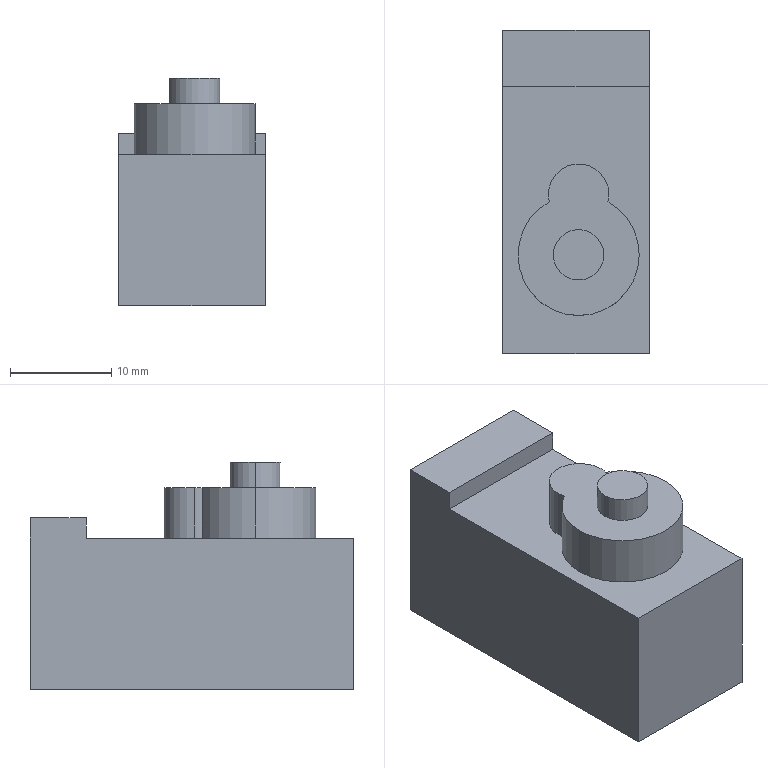Part | SolidWorks | features BaseBody 1 | 1 solid | 18 faces | box 14.483 x 32 x 22.5 mm | volume 7805 mm3 | plane 10 | cylinder 8 | commonest cylinder face diameters 6 x3 12 x3 5 x2
STEP:
#1=CARTESIAN_POINT('',(4.506,-11.764,22.5));
#2=VERTEX_POINT('',#1);
#3=CARTESIAN_POINT('',(-0.4937,-11.764,22.5));
#4=VERTEX_POINT('',#3);
#5=CARTESIAN_POINT('',(2.006,-11.764,22.5));
#6=DIRECTION('',(0.,0.,1.));
#7=DIRECTION('',(1.,0.,0.));
#8=AXIS2_PLACEMENT_3D('',#5,#6,#7);
#9=CIRCLE('',#8,2.5);
#10=EDGE_CURVE('',#2,#4,#9,.T.);
#11=ORIENTED_EDGE('',*,*,#10,.F.);
#12=CARTESIAN_POINT('',(4.506,-11.764,20.));
#13=VERTEX_POINT('',#12);
#14=CARTESIAN_POINT('',(4.506,-11.764,22.5));
#15=DIRECTION('',(0.,0.,-1.));
#16=VECTOR('',#15,1000.);
#17=LINE('',#14,#16);
#18=EDGE_CURVE('',#2,#13,#17,.T.);
#19=ORIENTED_EDGE('',*,*,#18,.T.);
#20=CARTESIAN_POINT('',(-0.4937,-11.764,20.));
#21=VERTEX_POINT('',#20);
#22=CARTESIAN_POINT('',(2.006,-11.764,20.));
#23=DIRECTION('',(0.,0.,1.));
#24=DIRECTION('',(1.,0.,0.));
#25=AXIS2_PLACEMENT_3D('',#22,#23,#24);
#26=CIRCLE('',#25,2.5);
#27=EDGE_CURVE('',#13,#21,#26,.T.);
#28=ORIENTED_EDGE('',*,*,#27,.T.);
#29=CARTESIAN_POINT('',(-0.4937,-11.764,22.5));
#30=DIRECTION('',(0.,0.,-1.));
#31=VECTOR('',#30,1000.);
#32=LINE('',#29,#31);
#33=EDGE_CURVE('',#4,#21,#32,.T.);
#34=ORIENTED_EDGE('',*,*,#33,.F.);
#35=EDGE_LOOP('',(#11,#19,#28,#34));
#36=FACE_OUTER_BOUND('',#35,.T.);
#37=CARTESIAN_POINT('',(2.006,-11.764,22.5));
#38=DIRECTION('',(0.,0.,-1.));
#39=DIRECTION('',(-1.,0.,0.));
#40=AXIS2_PLACEMENT_3D('',#37,#38,#39);
#41=CYLINDRICAL_SURFACE('',#40,2.5);
#42=ADVANCED_FACE('',(#36),#41,.T.);
#43=CARTESIAN_POINT('',(8.006,-11.764,20.));
#44=VERTEX_POINT('',#43);
#45=CARTESIAN_POINT('',(4.911,-6.514,20.));
#46=VERTEX_POINT('',#45);
#47=CARTESIAN_POINT('',(2.006,-11.764,20.));
#48=DIRECTION('',(0.,0.,1.));
#49=DIRECTION('',(1.,0.,0.));
#50=AXIS2_PLACEMENT_3D('',#47,#48,#49);
#51=CIRCLE('',#50,6.);
#52=EDGE_CURVE('',#44,#46,#51,.T.);
#53=ORIENTED_EDGE('',*,*,#52,.F.);
#54=CARTESIAN_POINT('',(8.006,-11.764,15.));
#55=VERTEX_POINT('',#54);
#56=CARTESIAN_POINT('',(8.006,-11.764,20.));
#57=DIRECTION('',(0.,0.,-1.));
#58=VECTOR('',#57,1000.);
#59=LINE('',#56,#58);
#60=EDGE_CURVE('',#44,#55,#59,.T.);
#61=ORIENTED_EDGE('',*,*,#60,.T.);
#62=CARTESIAN_POINT('',(4.911,-6.514,15.));
#63=VERTEX_POINT('',#62);
#64=CARTESIAN_POINT('',(2.006,-11.764,15.));
#65=DIRECTION('',(0.,0.,1.));
#66=DIRECTION('',(1.,0.,0.));
#67=AXIS2_PLACEMENT_3D('',#64,#65,#66);
#68=CIRCLE('',#67,6.);
#69=EDGE_CURVE('',#55,#63,#68,.T.);
#70=ORIENTED_EDGE('',*,*,#69,.T.);
#71=CARTESIAN_POINT('',(4.911,-6.514,20.));
#72=DIRECTION('',(0.,0.,-1.));
#73=VECTOR('',#72,1000.);
#74=LINE('',#71,#73);
#75=EDGE_CURVE('',#46,#63,#74,.T.);
#76=ORIENTED_EDGE('',*,*,#75,.F.);
#77=EDGE_LOOP('',(#53,#61,#70,#76));
#78=FACE_OUTER_BOUND('',#77,.T.);
#79=CARTESIAN_POINT('',(2.006,-11.764,20.));
#80=DIRECTION('',(0.,0.,-1.));
#81=DIRECTION('',(-1.,0.,0.));
#82=AXIS2_PLACEMENT_3D('',#79,#80,#81);
#83=CYLINDRICAL_SURFACE('',#82,6.);
#84=ADVANCED_FACE('',(#78),#83,.T.);
#85=ORIENTED_EDGE('',*,*,#60,.F.);
#86=CARTESIAN_POINT('',(-3.994,-11.764,20.));
#87=VERTEX_POINT('',#86);
#88=CARTESIAN_POINT('',(2.006,-11.764,20.));
#89=DIRECTION('',(0.,0.,1.));
#90=DIRECTION('',(1.,0.,0.));
#91=AXIS2_PLACEMENT_3D('',#88,#89,#90);
#92=CIRCLE('',#91,6.);
#93=EDGE_CURVE('',#87,#44,#92,.T.);
#94=ORIENTED_EDGE('',*,*,#93,.F.);
#95=CARTESIAN_POINT('',(-3.994,-11.764,15.));
#96=VERTEX_POINT('',#95);
#97=CARTESIAN_POINT('',(-3.994,-11.764,20.));
#98=DIRECTION('',(0.,0.,-1.));
#99=VECTOR('',#98,1000.);
#100=LINE('',#97,#99);
#101=EDGE_CURVE('',#87,#96,#100,.T.);
#102=ORIENTED_EDGE('',*,*,#101,.T.);
#103=CARTESIAN_POINT('',(2.006,-11.764,15.));
#104=DIRECTION('',(0.,0.,1.));
#105=DIRECTION('',(1.,0.,0.));
#106=AXIS2_PLACEMENT_3D('',#103,#104,#105);
#107=CIRCLE('',#106,6.);
#108=EDGE_CURVE('',#96,#55,#107,.T.);
#109=ORIENTED_EDGE('',*,*,#108,.T.);
#110=EDGE_LOOP('',(#85,#94,#102,#109));
#111=FACE_OUTER_BOUND('',#110,.T.);
#112=CARTESIAN_POINT('',(2.006,-11.764,20.));
#113=DIRECTION('',(0.,0.,-1.));
#114=DIRECTION('',(-1.,0.,0.));
#115=AXIS2_PLACEMENT_3D('',#112,#113,#114);
#116=CYLINDRICAL_SURFACE('',#115,6.);
#117=ADVANCED_FACE('',(#111),#116,.T.);
#118=CARTESIAN_POINT('',(5.006,-5.764,20.));
#119=VERTEX_POINT('',#118);
#120=CARTESIAN_POINT('',(-0.9937,-5.764,20.));
#121=VERTEX_POINT('',#120);
#122=CARTESIAN_POINT('',(2.006,-5.764,20.));
#123=DIRECTION('',(0.,0.,1.));
#124=DIRECTION('',(1.,0.,0.));
#125=AXIS2_PLACEMENT_3D('',#122,#123,#124);
#126=CIRCLE('',#125,3.);
#127=EDGE_CURVE('',#119,#121,#126,.T.);
#128=ORIENTED_EDGE('',*,*,#127,.F.);
#129=CARTESIAN_POINT('',(5.006,-5.764,15.));
#130=VERTEX_POINT('',#129);
#131=CARTESIAN_POINT('',(5.006,-5.764,20.));
#132=DIRECTION('',(0.,0.,-1.));
#133=VECTOR('',#132,1000.);
#134=LINE('',#131,#133);
#135=EDGE_CURVE('',#119,#130,#134,.T.);
#136=ORIENTED_EDGE('',*,*,#135,.T.);
#137=CARTESIAN_POINT('',(-0.9937,-5.764,15.));
#138=VERTEX_POINT('',#137);
#139=CARTESIAN_POINT('',(2.006,-5.764,15.));
#140=DIRECTION('',(0.,0.,1.));
#141=DIRECTION('',(1.,0.,0.));
#142=AXIS2_PLACEMENT_3D('',#139,#140,#141);
#143=CIRCLE('',#142,3.);
#144=EDGE_CURVE('',#130,#138,#143,.T.);
#145=ORIENTED_EDGE('',*,*,#144,.T.);
#146=CARTESIAN_POINT('',(-0.9937,-5.764,20.));
#147=DIRECTION('',(0.,0.,-1.));
#148=VECTOR('',#147,1000.);
#149=LINE('',#146,#148);
#150=EDGE_CURVE('',#121,#138,#149,.T.);
#151=ORIENTED_EDGE('',*,*,#150,.F.);
#152=EDGE_LOOP('',(#128,#136,#145,#151));
#153=FACE_OUTER_BOUND('',#152,.T.);
#154=CARTESIAN_POINT('',(2.006,-5.764,20.));
#155=DIRECTION('',(0.,0.,-1.));
#156=DIRECTION('',(-1.,0.,0.));
#157=AXIS2_PLACEMENT_3D('',#154,#155,#156);
#158=CYLINDRICAL_SURFACE('',#157,3.);
#159=ADVANCED_FACE('',(#153),#158,.T.);
#160=CARTESIAN_POINT('',(-0.8985,-6.514,20.));
#161=VERTEX_POINT('',#160);
#162=CARTESIAN_POINT('',(2.006,-5.764,20.));
#163=DIRECTION('',(0.,0.,1.));
#164=DIRECTION('',(1.,0.,0.));
#165=AXIS2_PLACEMENT_3D('',#162,#163,#164);
#166=CIRCLE('',#165,3.);
#167=EDGE_CURVE('',#121,#161,#166,.T.);
#168=ORIENTED_EDGE('',*,*,#167,.F.);
#169=ORIENTED_EDGE('',*,*,#150,.T.);
#170=CARTESIAN_POINT('',(-0.8985,-6.514,15.));
#171=VERTEX_POINT('',#170);
#172=CARTESIAN_POINT('',(2.006,-5.764,15.));
#173=DIRECTION('',(0.,0.,1.));
#174=DIRECTION('',(1.,0.,0.));
#175=AXIS2_PLACEMENT_3D('',#172,#173,#174);
#176=CIRCLE('',#175,3.);
#177=EDGE_CURVE('',#138,#171,#176,.T.);
#178=ORIENTED_EDGE('',*,*,#177,.T.);
#179=CARTESIAN_POINT('',(-0.8985,-6.514,20.));
#180=DIRECTION('',(0.,0.,-1.));
#181=VECTOR('',#180,1000.);
#182=LINE('',#179,#181);
#183=EDGE_CURVE('',#161,#171,#182,.T.);
#184=ORIENTED_EDGE('',*,*,#183,.F.);
#185=EDGE_LOOP('',(#168,#169,#178,#184));
#186=FACE_OUTER_BOUND('',#185,.T.);
#187=CARTESIAN_POINT('',(2.006,-5.764,20.));
#188=DIRECTION('',(0.,0.,-1.));
#189=DIRECTION('',(-1.,0.,0.));
#190=AXIS2_PLACEMENT_3D('',#187,#188,#189);
#191=CYLINDRICAL_SURFACE('',#190,3.);
#192=ADVANCED_FACE('',(#186),#191,.T.);
#193=CARTESIAN_POINT('',(-5.494,10.486,17.));
#194=VERTEX_POINT('',#193);
#195=CARTESIAN_POINT('',(-5.494,10.486,0.));
#196=VERTEX_POINT('',#195);
#197=CARTESIAN_POINT('',(-5.494,10.486,15.));
#198=DIRECTION('',(0.,0.,-1.));
#199=VECTOR('',#198,1000.);
#200=LINE('',#197,#199);
#201=EDGE_CURVE('',#194,#196,#200,.T.);
#202=ORIENTED_EDGE('',*,*,#201,.F.);
#203=CARTESIAN_POINT('',(8.99,10.486,17.));
#204=VERTEX_POINT('',#203);
#205=CARTESIAN_POINT('',(-5.494,10.486,17.));
#206=DIRECTION('',(-1.,0.,0.));
#207=VECTOR('',#206,1000.);
#208=LINE('',#205,#207);
#209=EDGE_CURVE('',#204,#194,#208,.T.);
#210=ORIENTED_EDGE('',*,*,#209,.F.);
#211=CARTESIAN_POINT('',(8.99,10.486,0.));
#212=VERTEX_POINT('',#211);
#213=CARTESIAN_POINT('',(8.99,10.486,15.));
#214=DIRECTION('',(0.,0.,-1.));
#215=VECTOR('',#214,1000.);
#216=LINE('',#213,#215);
#217=EDGE_CURVE('',#204,#212,#216,.T.);
#218=ORIENTED_EDGE('',*,*,#217,.T.);
#219=CARTESIAN_POINT('',(-5.494,10.486,0.));
#220=DIRECTION('',(-1.,0.,0.));
#221=VECTOR('',#220,1000.);
#222=LINE('',#219,#221);
#223=EDGE_CURVE('',#212,#196,#222,.T.);
#224=ORIENTED_EDGE('',*,*,#223,.T.);
#225=EDGE_LOOP('',(#202,#210,#218,#224));
#226=FACE_OUTER_BOUND('',#225,.T.);
#227=CARTESIAN_POINT('',(-5.494,10.486,15.));
#228=DIRECTION('',(0.,-1.,0.));
#229=DIRECTION('',(0.,0.,-1.));
#230=AXIS2_PLACEMENT_3D('',#227,#228,#229);
#231=PLANE('',#230);
#232=ADVANCED_FACE('',(#226),#231,.F.);
#233=CARTESIAN_POINT('',(-5.494,4.954,15.));
#234=VERTEX_POINT('',#233);
#235=CARTESIAN_POINT('',(-5.494,-21.514,15.));
#236=VERTEX_POINT('',#235);
#237=CARTESIAN_POINT('',(-5.494,10.486,15.));
#238=DIRECTION('',(0.,-1.,0.));
#239=VECTOR('',#238,1000.);
#240=LINE('',#237,#239);
#241=EDGE_CURVE('',#234,#236,#240,.T.);
#242=ORIENTED_EDGE('',*,*,#241,.F.);
#243=CARTESIAN_POINT('',(-5.494,4.954,17.));
#244=VERTEX_POINT('',#243);
#245=CARTESIAN_POINT('',(-5.494,4.954,17.));
#246=DIRECTION('',(0.,0.,-1.));
#247=VECTOR('',#246,1000.);
#248=LINE('',#245,#247);
#249=EDGE_CURVE('',#244,#234,#248,.T.);
#250=ORIENTED_EDGE('',*,*,#249,.F.);
#251=CARTESIAN_POINT('',(-5.494,10.486,17.));
#252=DIRECTION('',(0.,-1.,0.));
#253=VECTOR('',#252,1000.);
#254=LINE('',#251,#253);
#255=EDGE_CURVE('',#194,#244,#254,.T.);
#256=ORIENTED_EDGE('',*,*,#255,.F.);
#257=ORIENTED_EDGE('',*,*,#201,.T.);
#258=CARTESIAN_POINT('',(-5.494,-21.514,0.));
#259=VERTEX_POINT('',#258);
#260=CARTESIAN_POINT('',(-5.494,10.486,0.));
#261=DIRECTION('',(0.,-1.,0.));
#262=VECTOR('',#261,1000.);
#263=LINE('',#260,#262);
#264=EDGE_CURVE('',#196,#259,#263,.T.);
#265=ORIENTED_EDGE('',*,*,#264,.T.);
#266=CARTESIAN_POINT('',(-5.494,-21.514,15.));
#267=DIRECTION('',(0.,0.,-1.));
#268=VECTOR('',#267,1000.);
#269=LINE('',#266,#268);
#270=EDGE_CURVE('',#236,#259,#269,.T.);
#271=ORIENTED_EDGE('',*,*,#270,.F.);
#272=EDGE_LOOP('',(#242,#250,#256,#257,#265,#271));
#273=FACE_OUTER_BOUND('',#272,.T.);
#274=CARTESIAN_POINT('',(-5.494,10.486,15.));
#275=DIRECTION('',(1.,0.,0.));
#276=DIRECTION('',(0.,1.,0.));
#277=AXIS2_PLACEMENT_3D('',#274,#275,#276);
#278=PLANE('',#277);
#279=ADVANCED_FACE('',(#273),#278,.F.);
#280=CARTESIAN_POINT('',(8.99,-21.514,0.));
#281=VERTEX_POINT('',#280);
#282=CARTESIAN_POINT('',(-5.494,-21.514,0.));
#283=DIRECTION('',(1.,0.,0.));
#284=VECTOR('',#283,1000.);
#285=LINE('',#282,#284);
#286=EDGE_CURVE('',#259,#281,#285,.T.);
#287=ORIENTED_EDGE('',*,*,#286,.T.);
#288=CARTESIAN_POINT('',(8.99,-21.514,15.));
#289=VERTEX_POINT('',#288);
#290=CARTESIAN_POINT('',(8.99,-21.514,15.));
#291=DIRECTION('',(0.,0.,1.));
#292=VECTOR('',#291,1000.);
#293=LINE('',#290,#292);
#294=EDGE_CURVE('',#281,#289,#293,.T.);
#295=ORIENTED_EDGE('',*,*,#294,.T.);
#296=CARTESIAN_POINT('',(-5.494,-21.514,15.));
#297=DIRECTION('',(1.,0.,0.));
#298=VECTOR('',#297,1000.);
#299=LINE('',#296,#298);
#300=EDGE_CURVE('',#236,#289,#299,.T.);
#301=ORIENTED_EDGE('',*,*,#300,.F.);
#302=ORIENTED_EDGE('',*,*,#270,.T.);
#303=EDGE_LOOP('',(#287,#295,#301,#302));
#304=FACE_OUTER_BOUND('',#303,.T.);
#305=CARTESIAN_POINT('',(-5.494,-21.514,15.));
#306=DIRECTION('',(0.,1.,0.));
#307=DIRECTION('',(0.,0.,1.));
#308=AXIS2_PLACEMENT_3D('',#305,#306,#307);
#309=PLANE('',#308);
#310=ADVANCED_FACE('',(#304),#309,.F.);
#311=CARTESIAN_POINT('',(8.99,4.954,15.));
#312=VERTEX_POINT('',#311);
#313=CARTESIAN_POINT('',(8.99,11.57,15.));
#314=DIRECTION('',(0.,-1.,0.));
#315=VECTOR('',#314,1000.);
#316=LINE('',#313,#315);
#317=EDGE_CURVE('',#312,#289,#316,.T.);
#318=ORIENTED_EDGE('',*,*,#317,.F.);
#319=CARTESIAN_POINT('',(0.,4.954,15.));
#320=DIRECTION('',(1.,0.,0.));
#321=VECTOR('',#320,1000.);
#322=LINE('',#319,#321);
#323=EDGE_CURVE('',#234,#312,#322,.T.);
#324=ORIENTED_EDGE('',*,*,#323,.F.);
#325=ORIENTED_EDGE('',*,*,#241,.T.);
#326=ORIENTED_EDGE('',*,*,#300,.T.);
#327=EDGE_LOOP('',(#318,#324,#325,#326));
#328=FACE_OUTER_BOUND('',#327,.T.);
#329=CARTESIAN_POINT('',(2.006,-11.764,15.));
#330=DIRECTION('',(0.,0.,1.));
#331=DIRECTION('',(1.,0.,0.));
#332=AXIS2_PLACEMENT_3D('',#329,#330,#331);
#333=CIRCLE('',#332,6.);
#334=EDGE_CURVE('',#171,#96,#333,.T.);
#335=ORIENTED_EDGE('',*,*,#334,.F.);
#336=ORIENTED_EDGE('',*,*,#177,.F.);
#337=ORIENTED_EDGE('',*,*,#144,.F.);
#338=CARTESIAN_POINT('',(2.006,-5.764,15.));
#339=DIRECTION('',(0.,0.,1.));
#340=DIRECTION('',(1.,0.,0.));
#341=AXIS2_PLACEMENT_3D('',#338,#339,#340);
#342=CIRCLE('',#341,3.);
#343=EDGE_CURVE('',#63,#130,#342,.T.);
#344=ORIENTED_EDGE('',*,*,#343,.F.);
#345=ORIENTED_EDGE('',*,*,#69,.F.);
#346=ORIENTED_EDGE('',*,*,#108,.F.);
#347=EDGE_LOOP('',(#335,#336,#337,#344,#345,#346));
#348=FACE_BOUND('',#347,.T.);
#349=CARTESIAN_POINT('',(0.,0.,15.));
#350=DIRECTION('',(0.,0.,1.));
#351=DIRECTION('',(1.,0.,0.));
#352=AXIS2_PLACEMENT_3D('',#349,#350,#351);
#353=PLANE('',#352);
#354=ADVANCED_FACE('',(#328,#348),#353,.T.);
#355=ORIENTED_EDGE('',*,*,#223,.F.);
#356=CARTESIAN_POINT('',(8.99,0.,0.));
#357=DIRECTION('',(0.,-1.,0.));
#358=VECTOR('',#357,1000.);
#359=LINE('',#356,#358);
#360=EDGE_CURVE('',#212,#281,#359,.T.);
#361=ORIENTED_EDGE('',*,*,#360,.T.);
#362=ORIENTED_EDGE('',*,*,#286,.F.);
#363=ORIENTED_EDGE('',*,*,#264,.F.);
#364=EDGE_LOOP('',(#355,#361,#362,#363));
#365=FACE_OUTER_BOUND('',#364,.T.);
#366=CARTESIAN_POINT('',(0.,0.,0.));
#367=DIRECTION('',(0.,0.,1.));
#368=DIRECTION('',(1.,0.,0.));
#369=AXIS2_PLACEMENT_3D('',#366,#367,#368);
#370=PLANE('',#369);
#371=ADVANCED_FACE('',(#365),#370,.F.);
#372=ORIENTED_EDGE('',*,*,#135,.F.);
#373=CARTESIAN_POINT('',(2.006,-5.764,20.));
#374=DIRECTION('',(0.,0.,1.));
#375=DIRECTION('',(1.,0.,0.));
#376=AXIS2_PLACEMENT_3D('',#373,#374,#375);
#377=CIRCLE('',#376,3.);
#378=EDGE_CURVE('',#46,#119,#377,.T.);
#379=ORIENTED_EDGE('',*,*,#378,.F.);
#380=ORIENTED_EDGE('',*,*,#75,.T.);
#381=ORIENTED_EDGE('',*,*,#343,.T.);
#382=EDGE_LOOP('',(#372,#379,#380,#381));
#383=FACE_OUTER_BOUND('',#382,.T.);
#384=CARTESIAN_POINT('',(2.006,-5.764,20.));
#385=DIRECTION('',(0.,0.,-1.));
#386=DIRECTION('',(-1.,0.,0.));
#387=AXIS2_PLACEMENT_3D('',#384,#385,#386);
#388=CYLINDRICAL_SURFACE('',#387,3.);
#389=ADVANCED_FACE('',(#383),#388,.T.);
#390=ORIENTED_EDGE('',*,*,#101,.F.);
#391=CARTESIAN_POINT('',(2.006,-11.764,20.));
#392=DIRECTION('',(0.,0.,1.));
#393=DIRECTION('',(1.,0.,0.));
#394=AXIS2_PLACEMENT_3D('',#391,#392,#393);
#395=CIRCLE('',#394,6.);
#396=EDGE_CURVE('',#161,#87,#395,.T.);
#397=ORIENTED_EDGE('',*,*,#396,.F.);
#398=ORIENTED_EDGE('',*,*,#183,.T.);
#399=ORIENTED_EDGE('',*,*,#334,.T.);
#400=EDGE_LOOP('',(#390,#397,#398,#399));
#401=FACE_OUTER_BOUND('',#400,.T.);
#402=CARTESIAN_POINT('',(2.006,-11.764,20.));
#403=DIRECTION('',(0.,0.,-1.));
#404=DIRECTION('',(-1.,0.,0.));
#405=AXIS2_PLACEMENT_3D('',#402,#403,#404);
#406=CYLINDRICAL_SURFACE('',#405,6.);
#407=ADVANCED_FACE('',(#401),#406,.T.);
#408=CARTESIAN_POINT('',(2.006,-11.764,20.));
#409=DIRECTION('',(0.,0.,1.));
#410=DIRECTION('',(1.,0.,0.));
#411=AXIS2_PLACEMENT_3D('',#408,#409,#410);
#412=CIRCLE('',#411,2.5);
#413=EDGE_CURVE('',#21,#13,#412,.T.);
#414=ORIENTED_EDGE('',*,*,#413,.F.);
#415=ORIENTED_EDGE('',*,*,#27,.F.);
#416=EDGE_LOOP('',(#414,#415));
#417=FACE_BOUND('',#416,.T.);
#418=ORIENTED_EDGE('',*,*,#378,.T.);
#419=ORIENTED_EDGE('',*,*,#127,.T.);
#420=ORIENTED_EDGE('',*,*,#167,.T.);
#421=ORIENTED_EDGE('',*,*,#396,.T.);
#422=ORIENTED_EDGE('',*,*,#93,.T.);
#423=ORIENTED_EDGE('',*,*,#52,.T.);
#424=EDGE_LOOP('',(#418,#419,#420,#421,#422,#423));
#425=FACE_OUTER_BOUND('',#424,.T.);
#426=CARTESIAN_POINT('',(2.006,-8.764,20.));
#427=DIRECTION('',(0.,0.,1.));
#428=DIRECTION('',(1.,0.,0.));
#429=AXIS2_PLACEMENT_3D('',#426,#427,#428);
#430=PLANE('',#429);
#431=ADVANCED_FACE('',(#417,#425),#430,.T.);
#432=CARTESIAN_POINT('',(2.006,-11.764,22.5));
#433=DIRECTION('',(0.,0.,1.));
#434=DIRECTION('',(1.,0.,0.));
#435=AXIS2_PLACEMENT_3D('',#432,#433,#434);
#436=CIRCLE('',#435,2.5);
#437=EDGE_CURVE('',#4,#2,#436,.T.);
#438=ORIENTED_EDGE('',*,*,#437,.T.);
#439=ORIENTED_EDGE('',*,*,#10,.T.);
#440=EDGE_LOOP('',(#438,#439));
#441=FACE_OUTER_BOUND('',#440,.T.);
#442=CARTESIAN_POINT('',(2.006,-11.764,22.5));
#443=DIRECTION('',(0.,0.,1.));
#444=DIRECTION('',(1.,0.,0.));
#445=AXIS2_PLACEMENT_3D('',#442,#443,#444);
#446=PLANE('',#445);
#447=ADVANCED_FACE('',(#441),#446,.T.);
#448=ORIENTED_EDGE('',*,*,#18,.F.);
#449=ORIENTED_EDGE('',*,*,#437,.F.);
#450=ORIENTED_EDGE('',*,*,#33,.T.);
#451=ORIENTED_EDGE('',*,*,#413,.T.);
#452=EDGE_LOOP('',(#448,#449,#450,#451));
#453=FACE_OUTER_BOUND('',#452,.T.);
#454=CARTESIAN_POINT('',(2.006,-11.764,22.5));
#455=DIRECTION('',(0.,0.,-1.));
#456=DIRECTION('',(-1.,0.,0.));
#457=AXIS2_PLACEMENT_3D('',#454,#455,#456);
#458=CYLINDRICAL_SURFACE('',#457,2.5);
#459=ADVANCED_FACE('',(#453),#458,.T.);
#460=ORIENTED_EDGE('',*,*,#360,.F.);
#461=ORIENTED_EDGE('',*,*,#217,.F.);
#462=CARTESIAN_POINT('',(8.99,4.954,17.));
#463=VERTEX_POINT('',#462);
#464=CARTESIAN_POINT('',(8.99,10.486,17.));
#465=DIRECTION('',(0.,1.,0.));
#466=VECTOR('',#465,1000.);
#467=LINE('',#464,#466);
#468=EDGE_CURVE('',#463,#204,#467,.T.);
#469=ORIENTED_EDGE('',*,*,#468,.F.);
#470=CARTESIAN_POINT('',(8.99,4.954,17.));
#471=DIRECTION('',(0.,0.,-1.));
#472=VECTOR('',#471,1000.);
#473=LINE('',#470,#472);
#474=EDGE_CURVE('',#463,#312,#473,.T.);
#475=ORIENTED_EDGE('',*,*,#474,.T.);
#476=ORIENTED_EDGE('',*,*,#317,.T.);
#477=ORIENTED_EDGE('',*,*,#294,.F.);
#478=EDGE_LOOP('',(#460,#461,#469,#475,#476,#477));
#479=FACE_OUTER_BOUND('',#478,.T.);
#480=CARTESIAN_POINT('',(8.99,11.57,-3.));
#481=DIRECTION('',(-1.,0.,0.));
#482=DIRECTION('',(0.,0.,1.));
#483=AXIS2_PLACEMENT_3D('',#480,#481,#482);
#484=PLANE('',#483);
#485=ADVANCED_FACE('',(#479),#484,.F.);
#486=ORIENTED_EDGE('',*,*,#323,.T.);
#487=ORIENTED_EDGE('',*,*,#474,.F.);
#488=CARTESIAN_POINT('',(-5.494,4.954,17.));
#489=DIRECTION('',(1.,0.,0.));
#490=VECTOR('',#489,1000.);
#491=LINE('',#488,#490);
#492=EDGE_CURVE('',#244,#463,#491,.T.);
#493=ORIENTED_EDGE('',*,*,#492,.F.);
#494=ORIENTED_EDGE('',*,*,#249,.T.);
#495=EDGE_LOOP('',(#486,#487,#493,#494));
#496=FACE_OUTER_BOUND('',#495,.T.);
#497=CARTESIAN_POINT('',(-5.494,4.954,17.));
#498=DIRECTION('',(0.,1.,0.));
#499=DIRECTION('',(0.,0.,1.));
#500=AXIS2_PLACEMENT_3D('',#497,#498,#499);
#501=PLANE('',#500);
#502=ADVANCED_FACE('',(#496),#501,.F.);
#503=ORIENTED_EDGE('',*,*,#255,.T.);
#504=ORIENTED_EDGE('',*,*,#492,.T.);
#505=ORIENTED_EDGE('',*,*,#468,.T.);
#506=ORIENTED_EDGE('',*,*,#209,.T.);
#507=EDGE_LOOP('',(#503,#504,#505,#506));
#508=FACE_OUTER_BOUND('',#507,.T.);
#509=CARTESIAN_POINT('',(0.,0.,17.));
#510=DIRECTION('',(0.,0.,1.));
#511=DIRECTION('',(1.,0.,0.));
#512=AXIS2_PLACEMENT_3D('',#509,#510,#511);
#513=PLANE('',#512);
#514=ADVANCED_FACE('',(#508),#513,.T.);
#515=CLOSED_SHELL('',(#42,#84,#117,#159,#192,#232,#279,#310,#354,#371,#389,#407,#431,#447,#459,#485,#502,#514));
#516=MANIFOLD_SOLID_BREP('',#515);
#517=CARTESIAN_POINT('',(0.,0.,0.));
#518=DIRECTION('',(0.,0.,1.));
#519=DIRECTION('',(1.,0.,0.));
#520=AXIS2_PLACEMENT_3D('',#517,#518,#519);
#521=(LENGTH_UNIT()NAMED_UNIT(*)SI_UNIT(.MILLI.,.METRE.));
#522=UNCERTAINTY_MEASURE_WITH_UNIT(LENGTH_MEASURE(0.00001),#521,'','');
#523=(NAMED_UNIT(*)PLANE_ANGLE_UNIT()SI_UNIT($,.RADIAN.));
#524=(NAMED_UNIT(*)SI_UNIT($,.STERADIAN.)SOLID_ANGLE_UNIT());
#525=(GEOMETRIC_REPRESENTATION_CONTEXT(3)GLOBAL_UNCERTAINTY_ASSIGNED_CONTEXT((#522))GLOBAL_UNIT_ASSIGNED_CONTEXT((#521,#523,#524))REPRESENTATION_CONTEXT('',''));
#526=ADVANCED_BREP_SHAPE_REPRESENTATION('',(#516,#520),#525);